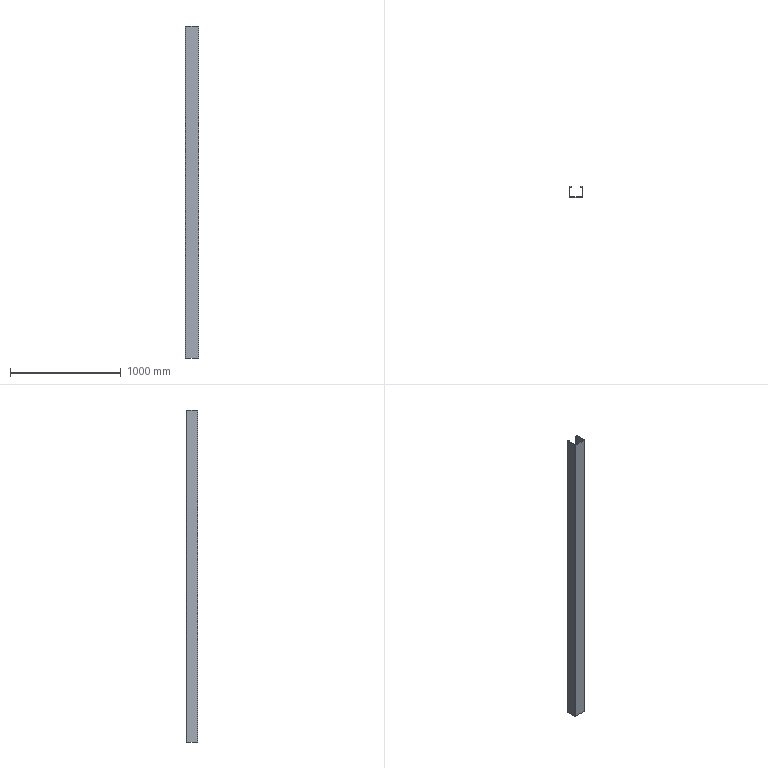Part | STEP file | SX-012-01 | 1 solid | 86 faces | box 120 x 100 x 2995 mm | volume 3086157 mm3 | plane 78 | cylinder 8 | commonest cylinder face diameters 0.4 x4 6.4 x4